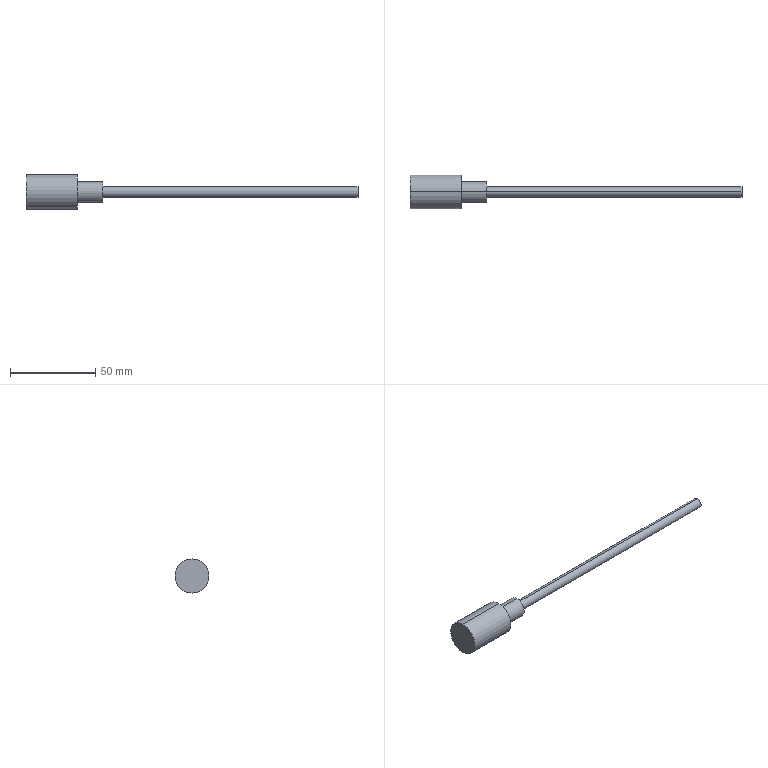Part | SolidWorks | features Revolution 1 | 1 solid | 10 faces | box 195 x 20 x 20 mm | volume 15362 mm3 | cylinder 6 | plane 4 | commonest cylinder face diameters 6 x2 12 x2 20 x2
STEP:
#1=CARTESIAN_POINT('',(195.,0.,3.));
#2=VERTEX_POINT('',#1);
#3=CARTESIAN_POINT('',(195.,0.,-3.));
#4=VERTEX_POINT('',#3);
#5=CARTESIAN_POINT('',(195.,0.,0.));
#6=DIRECTION('',(-1.,0.,0.));
#7=DIRECTION('',(0.,0.,1.));
#8=AXIS2_PLACEMENT_3D('',#5,#6,#7);
#9=CIRCLE('',#8,3.);
#10=EDGE_CURVE('',#2,#4,#9,.T.);
#11=ORIENTED_EDGE('',*,*,#10,.T.);
#12=CARTESIAN_POINT('',(45.,0.,-3.));
#13=VERTEX_POINT('',#12);
#14=CARTESIAN_POINT('',(0.,0.,-3.));
#15=DIRECTION('',(-1.,0.,0.));
#16=VECTOR('',#15,1000.);
#17=LINE('',#14,#16);
#18=EDGE_CURVE('',#4,#13,#17,.T.);
#19=ORIENTED_EDGE('',*,*,#18,.T.);
#20=CARTESIAN_POINT('',(45.,0.,3.));
#21=VERTEX_POINT('',#20);
#22=CARTESIAN_POINT('',(45.,0.,0.));
#23=DIRECTION('',(-1.,0.,0.));
#24=DIRECTION('',(0.,0.,1.));
#25=AXIS2_PLACEMENT_3D('',#22,#23,#24);
#26=CIRCLE('',#25,3.);
#27=EDGE_CURVE('',#21,#13,#26,.T.);
#28=ORIENTED_EDGE('',*,*,#27,.F.);
#29=CARTESIAN_POINT('',(0.,0.,3.));
#30=DIRECTION('',(-1.,0.,0.));
#31=VECTOR('',#30,1000.);
#32=LINE('',#29,#31);
#33=EDGE_CURVE('',#2,#21,#32,.T.);
#34=ORIENTED_EDGE('',*,*,#33,.F.);
#35=EDGE_LOOP('',(#11,#19,#28,#34));
#36=FACE_OUTER_BOUND('',#35,.T.);
#37=CARTESIAN_POINT('',(0.,0.,0.));
#38=DIRECTION('',(-1.,0.,0.));
#39=DIRECTION('',(0.,0.,1.));
#40=AXIS2_PLACEMENT_3D('',#37,#38,#39);
#41=CYLINDRICAL_SURFACE('',#40,3.);
#42=ADVANCED_FACE('',(#36),#41,.T.);
#43=CARTESIAN_POINT('',(45.,0.,6.));
#44=VERTEX_POINT('',#43);
#45=CARTESIAN_POINT('',(45.,0.,-6.));
#46=VERTEX_POINT('',#45);
#47=CARTESIAN_POINT('',(45.,0.,0.));
#48=DIRECTION('',(-1.,0.,0.));
#49=DIRECTION('',(0.,0.,1.));
#50=AXIS2_PLACEMENT_3D('',#47,#48,#49);
#51=CIRCLE('',#50,6.);
#52=EDGE_CURVE('',#44,#46,#51,.T.);
#53=ORIENTED_EDGE('',*,*,#52,.T.);
#54=CARTESIAN_POINT('',(30.,0.,-6.));
#55=VERTEX_POINT('',#54);
#56=CARTESIAN_POINT('',(0.,0.,-6.));
#57=DIRECTION('',(-1.,0.,0.));
#58=VECTOR('',#57,1000.);
#59=LINE('',#56,#58);
#60=EDGE_CURVE('',#46,#55,#59,.T.);
#61=ORIENTED_EDGE('',*,*,#60,.T.);
#62=CARTESIAN_POINT('',(30.,0.,6.));
#63=VERTEX_POINT('',#62);
#64=CARTESIAN_POINT('',(30.,0.,0.));
#65=DIRECTION('',(-1.,0.,0.));
#66=DIRECTION('',(0.,0.,1.));
#67=AXIS2_PLACEMENT_3D('',#64,#65,#66);
#68=CIRCLE('',#67,6.);
#69=EDGE_CURVE('',#63,#55,#68,.T.);
#70=ORIENTED_EDGE('',*,*,#69,.F.);
#71=CARTESIAN_POINT('',(0.,0.,6.));
#72=DIRECTION('',(-1.,0.,0.));
#73=VECTOR('',#72,1000.);
#74=LINE('',#71,#73);
#75=EDGE_CURVE('',#44,#63,#74,.T.);
#76=ORIENTED_EDGE('',*,*,#75,.F.);
#77=EDGE_LOOP('',(#53,#61,#70,#76));
#78=FACE_OUTER_BOUND('',#77,.T.);
#79=CARTESIAN_POINT('',(0.,0.,0.));
#80=DIRECTION('',(-1.,0.,0.));
#81=DIRECTION('',(0.,0.,1.));
#82=AXIS2_PLACEMENT_3D('',#79,#80,#81);
#83=CYLINDRICAL_SURFACE('',#82,6.);
#84=ADVANCED_FACE('',(#78),#83,.T.);
#85=CARTESIAN_POINT('',(30.,0.,10.));
#86=VERTEX_POINT('',#85);
#87=CARTESIAN_POINT('',(30.,0.,-10.));
#88=VERTEX_POINT('',#87);
#89=CARTESIAN_POINT('',(30.,0.,0.));
#90=DIRECTION('',(-1.,0.,0.));
#91=DIRECTION('',(0.,0.,1.));
#92=AXIS2_PLACEMENT_3D('',#89,#90,#91);
#93=CIRCLE('',#92,10.);
#94=EDGE_CURVE('',#86,#88,#93,.T.);
#95=ORIENTED_EDGE('',*,*,#94,.T.);
#96=CARTESIAN_POINT('',(0.,0.,-10.));
#97=VERTEX_POINT('',#96);
#98=CARTESIAN_POINT('',(0.,0.,-10.));
#99=DIRECTION('',(-1.,0.,0.));
#100=VECTOR('',#99,1000.);
#101=LINE('',#98,#100);
#102=EDGE_CURVE('',#88,#97,#101,.T.);
#103=ORIENTED_EDGE('',*,*,#102,.T.);
#104=CARTESIAN_POINT('',(0.,0.,10.));
#105=VERTEX_POINT('',#104);
#106=CARTESIAN_POINT('',(0.,0.,0.));
#107=DIRECTION('',(-1.,0.,0.));
#108=DIRECTION('',(0.,0.,1.));
#109=AXIS2_PLACEMENT_3D('',#106,#107,#108);
#110=CIRCLE('',#109,10.);
#111=EDGE_CURVE('',#105,#97,#110,.T.);
#112=ORIENTED_EDGE('',*,*,#111,.F.);
#113=CARTESIAN_POINT('',(0.,0.,10.));
#114=DIRECTION('',(-1.,0.,0.));
#115=VECTOR('',#114,1000.);
#116=LINE('',#113,#115);
#117=EDGE_CURVE('',#86,#105,#116,.T.);
#118=ORIENTED_EDGE('',*,*,#117,.F.);
#119=EDGE_LOOP('',(#95,#103,#112,#118));
#120=FACE_OUTER_BOUND('',#119,.T.);
#121=CARTESIAN_POINT('',(0.,0.,0.));
#122=DIRECTION('',(-1.,0.,0.));
#123=DIRECTION('',(0.,0.,1.));
#124=AXIS2_PLACEMENT_3D('',#121,#122,#123);
#125=CYLINDRICAL_SURFACE('',#124,10.);
#126=ADVANCED_FACE('',(#120),#125,.T.);
#127=ORIENTED_EDGE('',*,*,#111,.T.);
#128=CARTESIAN_POINT('',(0.,0.,0.));
#129=DIRECTION('',(-1.,0.,0.));
#130=DIRECTION('',(0.,0.,1.));
#131=AXIS2_PLACEMENT_3D('',#128,#129,#130);
#132=CIRCLE('',#131,10.);
#133=EDGE_CURVE('',#97,#105,#132,.T.);
#134=ORIENTED_EDGE('',*,*,#133,.T.);
#135=EDGE_LOOP('',(#127,#134));
#136=FACE_OUTER_BOUND('',#135,.T.);
#137=CARTESIAN_POINT('',(0.,0.,0.));
#138=DIRECTION('',(1.,0.,0.));
#139=DIRECTION('',(0.,0.,-1.));
#140=AXIS2_PLACEMENT_3D('',#137,#138,#139);
#141=PLANE('',#140);
#142=ADVANCED_FACE('',(#136),#141,.F.);
#143=ORIENTED_EDGE('',*,*,#102,.F.);
#144=CARTESIAN_POINT('',(30.,0.,0.));
#145=DIRECTION('',(-1.,0.,0.));
#146=DIRECTION('',(0.,0.,1.));
#147=AXIS2_PLACEMENT_3D('',#144,#145,#146);
#148=CIRCLE('',#147,10.);
#149=EDGE_CURVE('',#88,#86,#148,.T.);
#150=ORIENTED_EDGE('',*,*,#149,.T.);
#151=ORIENTED_EDGE('',*,*,#117,.T.);
#152=ORIENTED_EDGE('',*,*,#133,.F.);
#153=EDGE_LOOP('',(#143,#150,#151,#152));
#154=FACE_OUTER_BOUND('',#153,.T.);
#155=CARTESIAN_POINT('',(0.,0.,0.));
#156=DIRECTION('',(-1.,0.,0.));
#157=DIRECTION('',(0.,0.,1.));
#158=AXIS2_PLACEMENT_3D('',#155,#156,#157);
#159=CYLINDRICAL_SURFACE('',#158,10.);
#160=ADVANCED_FACE('',(#154),#159,.T.);
#161=ORIENTED_EDGE('',*,*,#94,.F.);
#162=ORIENTED_EDGE('',*,*,#149,.F.);
#163=EDGE_LOOP('',(#161,#162));
#164=FACE_OUTER_BOUND('',#163,.T.);
#165=ORIENTED_EDGE('',*,*,#69,.T.);
#166=CARTESIAN_POINT('',(30.,0.,0.));
#167=DIRECTION('',(-1.,0.,0.));
#168=DIRECTION('',(0.,0.,1.));
#169=AXIS2_PLACEMENT_3D('',#166,#167,#168);
#170=CIRCLE('',#169,6.);
#171=EDGE_CURVE('',#55,#63,#170,.T.);
#172=ORIENTED_EDGE('',*,*,#171,.T.);
#173=EDGE_LOOP('',(#165,#172));
#174=FACE_BOUND('',#173,.T.);
#175=CARTESIAN_POINT('',(30.,10.,0.));
#176=DIRECTION('',(-1.,0.,0.));
#177=DIRECTION('',(0.,0.,1.));
#178=AXIS2_PLACEMENT_3D('',#175,#176,#177);
#179=PLANE('',#178);
#180=ADVANCED_FACE('',(#164,#174),#179,.F.);
#181=ORIENTED_EDGE('',*,*,#60,.F.);
#182=CARTESIAN_POINT('',(45.,0.,0.));
#183=DIRECTION('',(-1.,0.,0.));
#184=DIRECTION('',(0.,0.,1.));
#185=AXIS2_PLACEMENT_3D('',#182,#183,#184);
#186=CIRCLE('',#185,6.);
#187=EDGE_CURVE('',#46,#44,#186,.T.);
#188=ORIENTED_EDGE('',*,*,#187,.T.);
#189=ORIENTED_EDGE('',*,*,#75,.T.);
#190=ORIENTED_EDGE('',*,*,#171,.F.);
#191=EDGE_LOOP('',(#181,#188,#189,#190));
#192=FACE_OUTER_BOUND('',#191,.T.);
#193=CARTESIAN_POINT('',(0.,0.,0.));
#194=DIRECTION('',(-1.,0.,0.));
#195=DIRECTION('',(0.,0.,1.));
#196=AXIS2_PLACEMENT_3D('',#193,#194,#195);
#197=CYLINDRICAL_SURFACE('',#196,6.);
#198=ADVANCED_FACE('',(#192),#197,.T.);
#199=ORIENTED_EDGE('',*,*,#52,.F.);
#200=ORIENTED_EDGE('',*,*,#187,.F.);
#201=EDGE_LOOP('',(#199,#200));
#202=FACE_OUTER_BOUND('',#201,.T.);
#203=ORIENTED_EDGE('',*,*,#27,.T.);
#204=CARTESIAN_POINT('',(45.,0.,0.));
#205=DIRECTION('',(-1.,0.,0.));
#206=DIRECTION('',(0.,0.,1.));
#207=AXIS2_PLACEMENT_3D('',#204,#205,#206);
#208=CIRCLE('',#207,3.);
#209=EDGE_CURVE('',#13,#21,#208,.T.);
#210=ORIENTED_EDGE('',*,*,#209,.T.);
#211=EDGE_LOOP('',(#203,#210));
#212=FACE_BOUND('',#211,.T.);
#213=CARTESIAN_POINT('',(45.,6.,0.));
#214=DIRECTION('',(-1.,0.,0.));
#215=DIRECTION('',(0.,0.,1.));
#216=AXIS2_PLACEMENT_3D('',#213,#214,#215);
#217=PLANE('',#216);
#218=ADVANCED_FACE('',(#202,#212),#217,.F.);
#219=ORIENTED_EDGE('',*,*,#18,.F.);
#220=CARTESIAN_POINT('',(195.,0.,0.));
#221=DIRECTION('',(-1.,0.,0.));
#222=DIRECTION('',(0.,0.,1.));
#223=AXIS2_PLACEMENT_3D('',#220,#221,#222);
#224=CIRCLE('',#223,3.);
#225=EDGE_CURVE('',#4,#2,#224,.T.);
#226=ORIENTED_EDGE('',*,*,#225,.T.);
#227=ORIENTED_EDGE('',*,*,#33,.T.);
#228=ORIENTED_EDGE('',*,*,#209,.F.);
#229=EDGE_LOOP('',(#219,#226,#227,#228));
#230=FACE_OUTER_BOUND('',#229,.T.);
#231=CARTESIAN_POINT('',(0.,0.,0.));
#232=DIRECTION('',(-1.,0.,0.));
#233=DIRECTION('',(0.,0.,1.));
#234=AXIS2_PLACEMENT_3D('',#231,#232,#233);
#235=CYLINDRICAL_SURFACE('',#234,3.);
#236=ADVANCED_FACE('',(#230),#235,.T.);
#237=ORIENTED_EDGE('',*,*,#10,.F.);
#238=ORIENTED_EDGE('',*,*,#225,.F.);
#239=EDGE_LOOP('',(#237,#238));
#240=FACE_OUTER_BOUND('',#239,.T.);
#241=CARTESIAN_POINT('',(195.,3.,0.));
#242=DIRECTION('',(-1.,0.,0.));
#243=DIRECTION('',(0.,0.,1.));
#244=AXIS2_PLACEMENT_3D('',#241,#242,#243);
#245=PLANE('',#244);
#246=ADVANCED_FACE('',(#240),#245,.F.);
#247=CLOSED_SHELL('',(#42,#84,#126,#142,#160,#180,#198,#218,#236,#246));
#248=MANIFOLD_SOLID_BREP('',#247);
#249=CARTESIAN_POINT('',(0.,0.,0.));
#250=DIRECTION('',(0.,0.,1.));
#251=DIRECTION('',(1.,0.,0.));
#252=AXIS2_PLACEMENT_3D('',#249,#250,#251);
#253=(LENGTH_UNIT()NAMED_UNIT(*)SI_UNIT(.MILLI.,.METRE.));
#254=UNCERTAINTY_MEASURE_WITH_UNIT(LENGTH_MEASURE(0.00001),#253,'','');
#255=(NAMED_UNIT(*)PLANE_ANGLE_UNIT()SI_UNIT($,.RADIAN.));
#256=(NAMED_UNIT(*)SI_UNIT($,.STERADIAN.)SOLID_ANGLE_UNIT());
#257=(GEOMETRIC_REPRESENTATION_CONTEXT(3)GLOBAL_UNCERTAINTY_ASSIGNED_CONTEXT((#254))GLOBAL_UNIT_ASSIGNED_CONTEXT((#253,#255,#256))REPRESENTATION_CONTEXT('',''));
#258=ADVANCED_BREP_SHAPE_REPRESENTATION('',(#248,#252),#257);